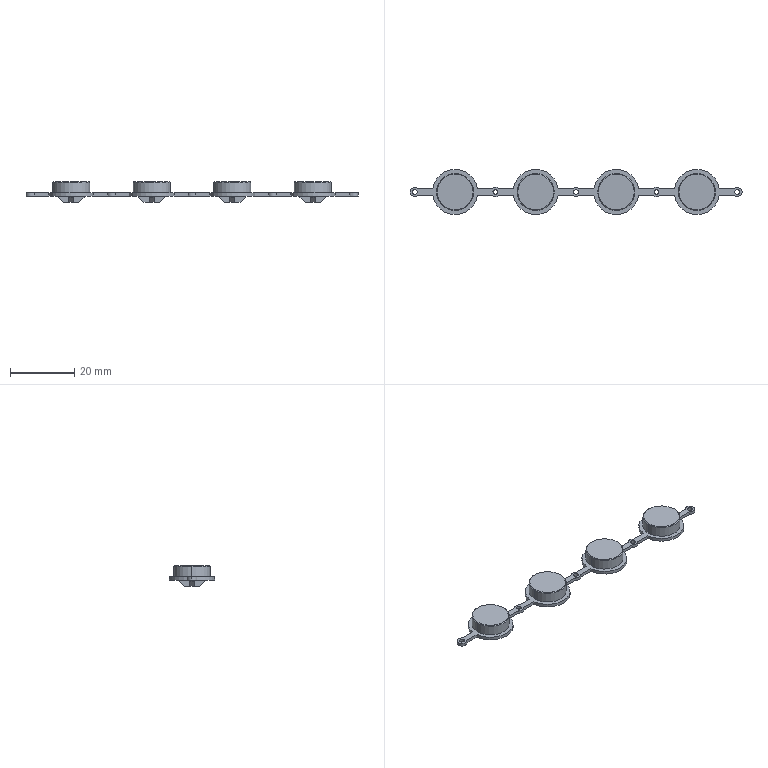Part | SolidWorks | features Chamfer 2, ICE 2, Extrusion 1 | 1 solid | 133 faces | box 103 x 14 x 6.5 mm | volume 2303 mm3 | plane 90 | cylinder 35 | cone 8 | commonest cylinder face diameters 1.5 x10 3 x9 11.5 x8 14 x8